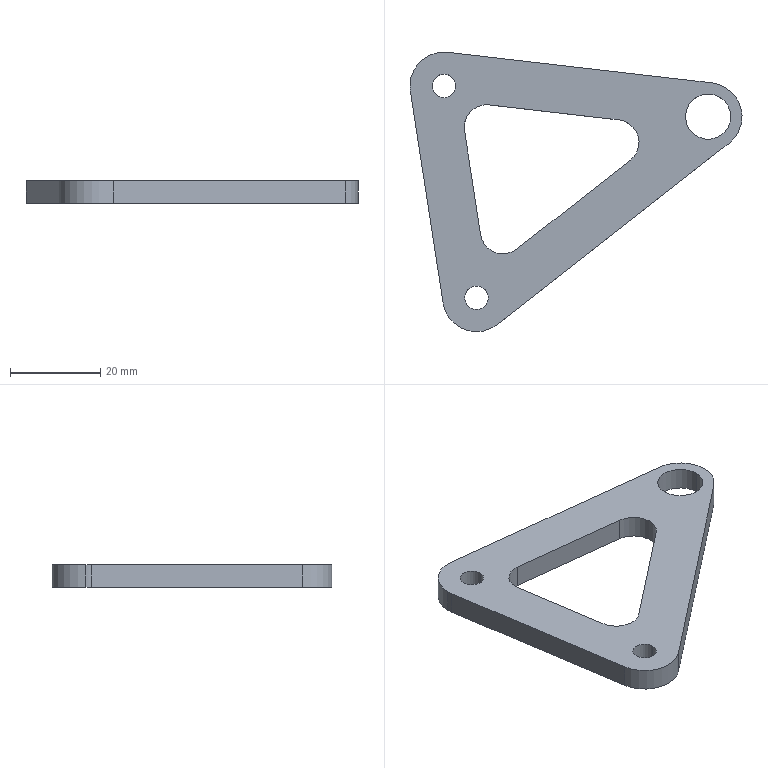Part | SolidWorks | features Extrusion 1 | 1 solid | 22 faces | box 73.414 x 61.829 x 5 mm | volume 9310 mm3 | cylinder 14 | plane 8 | commonest cylinder face diameters 10 x6 5.2 x4 15 x4
STEP:
#1=CARTESIAN_POINT('',(10.08,-4.188,5.));
#2=VERTEX_POINT('',#1);
#3=CARTESIAN_POINT('',(4.505,-9.155,5.));
#4=VERTEX_POINT('',#3);
#5=CARTESIAN_POINT('',(9.505,-9.155,5.));
#6=DIRECTION('',(0.,0.,1.));
#7=DIRECTION('',(-1.,0.,0.));
#8=AXIS2_PLACEMENT_3D('',#5,#6,#7);
#9=CIRCLE('',#8,5.);
#10=EDGE_CURVE('',#2,#4,#9,.T.);
#11=ORIENTED_EDGE('',*,*,#10,.T.);
#12=CARTESIAN_POINT('',(4.505,-9.155,0.));
#13=VERTEX_POINT('',#12);
#14=CARTESIAN_POINT('',(4.505,-9.155,5.));
#15=DIRECTION('',(0.,0.,-1.));
#16=VECTOR('',#15,1000.);
#17=LINE('',#14,#16);
#18=EDGE_CURVE('',#4,#13,#17,.T.);
#19=ORIENTED_EDGE('',*,*,#18,.T.);
#20=CARTESIAN_POINT('',(10.08,-4.188,0.));
#21=VERTEX_POINT('',#20);
#22=CARTESIAN_POINT('',(9.505,-9.155,0.));
#23=DIRECTION('',(0.,0.,1.));
#24=DIRECTION('',(-1.,0.,0.));
#25=AXIS2_PLACEMENT_3D('',#22,#23,#24);
#26=CIRCLE('',#25,5.);
#27=EDGE_CURVE('',#21,#13,#26,.T.);
#28=ORIENTED_EDGE('',*,*,#27,.F.);
#29=CARTESIAN_POINT('',(10.08,-4.188,5.));
#30=DIRECTION('',(0.,0.,-1.));
#31=VECTOR('',#30,1000.);
#32=LINE('',#29,#31);
#33=EDGE_CURVE('',#2,#21,#32,.T.);
#34=ORIENTED_EDGE('',*,*,#33,.F.);
#35=EDGE_LOOP('',(#11,#19,#28,#34));
#36=FACE_OUTER_BOUND('',#35,.T.);
#37=CARTESIAN_POINT('',(9.505,-9.155,5.));
#38=DIRECTION('',(0.,0.,-1.));
#39=DIRECTION('',(-1.,0.,0.));
#40=AXIS2_PLACEMENT_3D('',#37,#38,#39);
#41=CYLINDRICAL_SURFACE('',#40,5.);
#42=ADVANCED_FACE('',(#36),#41,.F.);
#43=CARTESIAN_POINT('',(-2.6,0.,5.));
#44=VERTEX_POINT('',#43);
#45=CARTESIAN_POINT('',(2.6,0.,5.));
#46=VERTEX_POINT('',#45);
#47=CARTESIAN_POINT('',(0.,0.,5.));
#48=DIRECTION('',(0.,0.,1.));
#49=DIRECTION('',(1.,0.,0.));
#50=AXIS2_PLACEMENT_3D('',#47,#48,#49);
#51=CIRCLE('',#50,2.6);
#52=EDGE_CURVE('',#44,#46,#51,.T.);
#53=ORIENTED_EDGE('',*,*,#52,.T.);
#54=CARTESIAN_POINT('',(2.6,0.,0.));
#55=VERTEX_POINT('',#54);
#56=CARTESIAN_POINT('',(2.6,0.,5.));
#57=DIRECTION('',(0.,0.,-1.));
#58=VECTOR('',#57,1000.);
#59=LINE('',#56,#58);
#60=EDGE_CURVE('',#46,#55,#59,.T.);
#61=ORIENTED_EDGE('',*,*,#60,.T.);
#62=CARTESIAN_POINT('',(-2.6,0.,0.));
#63=VERTEX_POINT('',#62);
#64=CARTESIAN_POINT('',(0.,0.,0.));
#65=DIRECTION('',(0.,0.,1.));
#66=DIRECTION('',(1.,0.,0.));
#67=AXIS2_PLACEMENT_3D('',#64,#65,#66);
#68=CIRCLE('',#67,2.6);
#69=EDGE_CURVE('',#63,#55,#68,.T.);
#70=ORIENTED_EDGE('',*,*,#69,.F.);
#71=CARTESIAN_POINT('',(-2.6,0.,5.));
#72=DIRECTION('',(0.,0.,-1.));
#73=VECTOR('',#72,1000.);
#74=LINE('',#71,#73);
#75=EDGE_CURVE('',#44,#63,#74,.T.);
#76=ORIENTED_EDGE('',*,*,#75,.F.);
#77=EDGE_LOOP('',(#53,#61,#70,#76));
#78=FACE_OUTER_BOUND('',#77,.T.);
#79=CARTESIAN_POINT('',(0.,0.,5.));
#80=DIRECTION('',(0.,0.,-1.));
#81=DIRECTION('',(-1.,0.,0.));
#82=AXIS2_PLACEMENT_3D('',#79,#80,#81);
#83=CYLINDRICAL_SURFACE('',#82,2.6);
#84=ADVANCED_FACE('',(#78),#83,.F.);
#85=CARTESIAN_POINT('',(53.414,-6.768,5.));
#86=VERTEX_POINT('',#85);
#87=CARTESIAN_POINT('',(63.414,-6.768,5.));
#88=VERTEX_POINT('',#87);
#89=CARTESIAN_POINT('',(58.414,-6.768,5.));
#90=DIRECTION('',(0.,0.,1.));
#91=DIRECTION('',(1.,0.,0.));
#92=AXIS2_PLACEMENT_3D('',#89,#90,#91);
#93=CIRCLE('',#92,5.);
#94=EDGE_CURVE('',#86,#88,#93,.T.);
#95=ORIENTED_EDGE('',*,*,#94,.T.);
#96=CARTESIAN_POINT('',(63.414,-6.768,0.));
#97=VERTEX_POINT('',#96);
#98=CARTESIAN_POINT('',(63.414,-6.768,5.));
#99=DIRECTION('',(0.,0.,-1.));
#100=VECTOR('',#99,1000.);
#101=LINE('',#98,#100);
#102=EDGE_CURVE('',#88,#97,#101,.T.);
#103=ORIENTED_EDGE('',*,*,#102,.T.);
#104=CARTESIAN_POINT('',(53.414,-6.768,0.));
#105=VERTEX_POINT('',#104);
#106=CARTESIAN_POINT('',(58.414,-6.768,0.));
#107=DIRECTION('',(0.,0.,1.));
#108=DIRECTION('',(1.,0.,0.));
#109=AXIS2_PLACEMENT_3D('',#106,#107,#108);
#110=CIRCLE('',#109,5.);
#111=EDGE_CURVE('',#105,#97,#110,.T.);
#112=ORIENTED_EDGE('',*,*,#111,.F.);
#113=CARTESIAN_POINT('',(53.414,-6.768,5.));
#114=DIRECTION('',(0.,0.,-1.));
#115=VECTOR('',#114,1000.);
#116=LINE('',#113,#115);
#117=EDGE_CURVE('',#86,#105,#116,.T.);
#118=ORIENTED_EDGE('',*,*,#117,.F.);
#119=EDGE_LOOP('',(#95,#103,#112,#118));
#120=FACE_OUTER_BOUND('',#119,.T.);
#121=CARTESIAN_POINT('',(58.414,-6.768,5.));
#122=DIRECTION('',(0.,0.,-1.));
#123=DIRECTION('',(-1.,0.,0.));
#124=AXIS2_PLACEMENT_3D('',#121,#122,#123);
#125=CYLINDRICAL_SURFACE('',#124,5.);
#126=ADVANCED_FACE('',(#120),#125,.F.);
#127=CARTESIAN_POINT('',(4.614,-46.829,5.));
#128=VERTEX_POINT('',#127);
#129=CARTESIAN_POINT('',(9.814,-46.829,5.));
#130=VERTEX_POINT('',#129);
#131=CARTESIAN_POINT('',(7.214,-46.829,5.));
#132=DIRECTION('',(0.,0.,1.));
#133=DIRECTION('',(1.,0.,0.));
#134=AXIS2_PLACEMENT_3D('',#131,#132,#133);
#135=CIRCLE('',#134,2.6);
#136=EDGE_CURVE('',#128,#130,#135,.T.);
#137=ORIENTED_EDGE('',*,*,#136,.T.);
#138=CARTESIAN_POINT('',(9.814,-46.829,0.));
#139=VERTEX_POINT('',#138);
#140=CARTESIAN_POINT('',(9.814,-46.829,5.));
#141=DIRECTION('',(0.,0.,-1.));
#142=VECTOR('',#141,1000.);
#143=LINE('',#140,#142);
#144=EDGE_CURVE('',#130,#139,#143,.T.);
#145=ORIENTED_EDGE('',*,*,#144,.T.);
#146=CARTESIAN_POINT('',(4.614,-46.829,0.));
#147=VERTEX_POINT('',#146);
#148=CARTESIAN_POINT('',(7.214,-46.829,0.));
#149=DIRECTION('',(0.,0.,1.));
#150=DIRECTION('',(1.,0.,0.));
#151=AXIS2_PLACEMENT_3D('',#148,#149,#150);
#152=CIRCLE('',#151,2.6);
#153=EDGE_CURVE('',#147,#139,#152,.T.);
#154=ORIENTED_EDGE('',*,*,#153,.F.);
#155=CARTESIAN_POINT('',(4.614,-46.829,5.));
#156=DIRECTION('',(0.,0.,-1.));
#157=VECTOR('',#156,1000.);
#158=LINE('',#155,#157);
#159=EDGE_CURVE('',#128,#147,#158,.T.);
#160=ORIENTED_EDGE('',*,*,#159,.F.);
#161=EDGE_LOOP('',(#137,#145,#154,#160));
#162=FACE_OUTER_BOUND('',#161,.T.);
#163=CARTESIAN_POINT('',(7.214,-46.829,5.));
#164=DIRECTION('',(0.,0.,-1.));
#165=DIRECTION('',(-1.,0.,0.));
#166=AXIS2_PLACEMENT_3D('',#163,#164,#165);
#167=CYLINDRICAL_SURFACE('',#166,2.6);
#168=ADVANCED_FACE('',(#162),#167,.F.);
#169=CARTESIAN_POINT('',(-7.5,0.,5.));
#170=VERTEX_POINT('',#169);
#171=CARTESIAN_POINT('',(-7.413,-1.142,5.));
#172=VERTEX_POINT('',#171);
#173=CARTESIAN_POINT('',(0.,0.,5.));
#174=DIRECTION('',(0.,0.,1.));
#175=DIRECTION('',(1.,0.,0.));
#176=AXIS2_PLACEMENT_3D('',#173,#174,#175);
#177=CIRCLE('',#176,7.5);
#178=EDGE_CURVE('',#170,#172,#177,.T.);
#179=ORIENTED_EDGE('',*,*,#178,.F.);
#180=CARTESIAN_POINT('',(-7.5,0.,0.));
#181=VERTEX_POINT('',#180);
#182=CARTESIAN_POINT('',(-7.5,0.,5.));
#183=DIRECTION('',(0.,0.,-1.));
#184=VECTOR('',#183,1000.);
#185=LINE('',#182,#184);
#186=EDGE_CURVE('',#170,#181,#185,.T.);
#187=ORIENTED_EDGE('',*,*,#186,.T.);
#188=CARTESIAN_POINT('',(-7.413,-1.142,0.));
#189=VERTEX_POINT('',#188);
#190=CARTESIAN_POINT('',(0.,0.,0.));
#191=DIRECTION('',(0.,0.,1.));
#192=DIRECTION('',(1.,0.,0.));
#193=AXIS2_PLACEMENT_3D('',#190,#191,#192);
#194=CIRCLE('',#193,7.5);
#195=EDGE_CURVE('',#181,#189,#194,.T.);
#196=ORIENTED_EDGE('',*,*,#195,.T.);
#197=CARTESIAN_POINT('',(-7.413,-1.142,5.));
#198=DIRECTION('',(0.,0.,-1.));
#199=VECTOR('',#198,1000.);
#200=LINE('',#197,#199);
#201=EDGE_CURVE('',#172,#189,#200,.T.);
#202=ORIENTED_EDGE('',*,*,#201,.F.);
#203=EDGE_LOOP('',(#179,#187,#196,#202));
#204=FACE_OUTER_BOUND('',#203,.T.);
#205=CARTESIAN_POINT('',(0.,0.,5.));
#206=DIRECTION('',(0.,0.,-1.));
#207=DIRECTION('',(-1.,0.,0.));
#208=AXIS2_PLACEMENT_3D('',#205,#206,#207);
#209=CYLINDRICAL_SURFACE('',#208,7.5);
#210=ADVANCED_FACE('',(#204),#209,.T.);
#211=ORIENTED_EDGE('',*,*,#94,.F.);
#212=CARTESIAN_POINT('',(58.414,-6.768,5.));
#213=DIRECTION('',(0.,0.,1.));
#214=DIRECTION('',(1.,0.,0.));
#215=AXIS2_PLACEMENT_3D('',#212,#213,#214);
#216=CIRCLE('',#215,5.);
#217=EDGE_CURVE('',#88,#86,#216,.T.);
#218=ORIENTED_EDGE('',*,*,#217,.F.);
#219=EDGE_LOOP('',(#211,#218));
#220=FACE_BOUND('',#219,.T.);
#221=CARTESIAN_POINT('',(63.036,-12.674,5.));
#222=VERTEX_POINT('',#221);
#223=CARTESIAN_POINT('',(59.277,0.6826,5.));
#224=VERTEX_POINT('',#223);
#225=CARTESIAN_POINT('',(58.414,-6.768,5.));
#226=DIRECTION('',(0.,0.,1.));
#227=DIRECTION('',(1.,0.,0.));
#228=AXIS2_PLACEMENT_3D('',#225,#226,#227);
#229=CIRCLE('',#228,7.5);
#230=EDGE_CURVE('',#222,#224,#229,.T.);
#231=ORIENTED_EDGE('',*,*,#230,.T.);
#232=CARTESIAN_POINT('',(0.8631,7.45,5.));
#233=VERTEX_POINT('',#232);
#234=CARTESIAN_POINT('',(59.277,0.6826,5.));
#235=DIRECTION('',(-0.9934,0.1151,0.));
#236=VECTOR('',#235,1000.);
#237=LINE('',#234,#236);
#238=EDGE_CURVE('',#224,#233,#237,.T.);
#239=ORIENTED_EDGE('',*,*,#238,.T.);
#240=CARTESIAN_POINT('',(0.,0.,5.));
#241=DIRECTION('',(0.,0.,1.));
#242=DIRECTION('',(1.,0.,0.));
#243=AXIS2_PLACEMENT_3D('',#240,#241,#242);
#244=CIRCLE('',#243,7.5);
#245=EDGE_CURVE('',#233,#170,#244,.T.);
#246=ORIENTED_EDGE('',*,*,#245,.T.);
#247=ORIENTED_EDGE('',*,*,#178,.T.);
#248=CARTESIAN_POINT('',(-0.1986,-47.971,5.));
#249=VERTEX_POINT('',#248);
#250=CARTESIAN_POINT('',(-7.413,-1.142,5.));
#251=DIRECTION('',(0.1523,-0.9883,0.));
#252=VECTOR('',#251,1000.);
#253=LINE('',#250,#252);
#254=EDGE_CURVE('',#172,#249,#253,.T.);
#255=ORIENTED_EDGE('',*,*,#254,.T.);
#256=CARTESIAN_POINT('',(11.836,-52.736,5.));
#257=VERTEX_POINT('',#256);
#258=CARTESIAN_POINT('',(7.214,-46.829,5.));
#259=DIRECTION('',(0.,0.,1.));
#260=DIRECTION('',(1.,0.,0.));
#261=AXIS2_PLACEMENT_3D('',#258,#259,#260);
#262=CIRCLE('',#261,7.5);
#263=EDGE_CURVE('',#249,#257,#262,.T.);
#264=ORIENTED_EDGE('',*,*,#263,.T.);
#265=CARTESIAN_POINT('',(11.836,-52.736,5.));
#266=DIRECTION('',(0.7876,0.6162,0.));
#267=VECTOR('',#266,1000.);
#268=LINE('',#265,#267);
#269=EDGE_CURVE('',#257,#222,#268,.T.);
#270=ORIENTED_EDGE('',*,*,#269,.T.);
#271=EDGE_LOOP('',(#231,#239,#246,#247,#255,#264,#270));
#272=FACE_OUTER_BOUND('',#271,.T.);
#273=ORIENTED_EDGE('',*,*,#136,.F.);
#274=CARTESIAN_POINT('',(7.214,-46.829,5.));
#275=DIRECTION('',(0.,0.,1.));
#276=DIRECTION('',(1.,0.,0.));
#277=AXIS2_PLACEMENT_3D('',#274,#275,#276);
#278=CIRCLE('',#277,2.6);
#279=EDGE_CURVE('',#130,#128,#278,.T.);
#280=ORIENTED_EDGE('',*,*,#279,.F.);
#281=EDGE_LOOP('',(#273,#280));
#282=FACE_BOUND('',#281,.T.);
#283=ORIENTED_EDGE('',*,*,#52,.F.);
#284=CARTESIAN_POINT('',(0.,0.,5.));
#285=DIRECTION('',(0.,0.,1.));
#286=DIRECTION('',(1.,0.,0.));
#287=AXIS2_PLACEMENT_3D('',#284,#285,#286);
#288=CIRCLE('',#287,2.6);
#289=EDGE_CURVE('',#46,#44,#288,.T.);
#290=ORIENTED_EDGE('',*,*,#289,.F.);
#291=EDGE_LOOP('',(#283,#290));
#292=FACE_BOUND('',#291,.T.);
#293=CARTESIAN_POINT('',(16.122,-36.05,5.));
#294=VERTEX_POINT('',#293);
#295=CARTESIAN_POINT('',(41.222,-16.41,5.));
#296=VERTEX_POINT('',#295);
#297=CARTESIAN_POINT('',(16.122,-36.05,5.));
#298=DIRECTION('',(0.7876,0.6162,0.));
#299=VECTOR('',#298,1000.);
#300=LINE('',#297,#299);
#301=EDGE_CURVE('',#294,#296,#300,.T.);
#302=ORIENTED_EDGE('',*,*,#301,.F.);
#303=CARTESIAN_POINT('',(8.099,-32.873,5.));
#304=VERTEX_POINT('',#303);
#305=CARTESIAN_POINT('',(13.041,-32.112,5.));
#306=DIRECTION('',(0.,0.,1.));
#307=DIRECTION('',(-1.,0.,0.));
#308=AXIS2_PLACEMENT_3D('',#305,#306,#307);
#309=CIRCLE('',#308,5.);
#310=EDGE_CURVE('',#304,#294,#309,.T.);
#311=ORIENTED_EDGE('',*,*,#310,.F.);
#312=CARTESIAN_POINT('',(4.563,-9.916,5.));
#313=VERTEX_POINT('',#312);
#314=CARTESIAN_POINT('',(4.563,-9.916,5.));
#315=DIRECTION('',(0.1523,-0.9883,0.));
#316=VECTOR('',#315,1000.);
#317=LINE('',#314,#316);
#318=EDGE_CURVE('',#313,#304,#317,.T.);
#319=ORIENTED_EDGE('',*,*,#318,.F.);
#320=CARTESIAN_POINT('',(9.505,-9.155,5.));
#321=DIRECTION('',(0.,0.,1.));
#322=DIRECTION('',(-1.,0.,0.));
#323=AXIS2_PLACEMENT_3D('',#320,#321,#322);
#324=CIRCLE('',#323,5.);
#325=EDGE_CURVE('',#4,#313,#324,.T.);
#326=ORIENTED_EDGE('',*,*,#325,.F.);
#327=ORIENTED_EDGE('',*,*,#10,.F.);
#328=CARTESIAN_POINT('',(38.717,-7.506,5.));
#329=VERTEX_POINT('',#328);
#330=CARTESIAN_POINT('',(38.717,-7.506,5.));
#331=DIRECTION('',(-0.9934,0.1151,0.));
#332=VECTOR('',#331,1000.);
#333=LINE('',#330,#332);
#334=EDGE_CURVE('',#329,#2,#333,.T.);
#335=ORIENTED_EDGE('',*,*,#334,.F.);
#336=CARTESIAN_POINT('',(38.141,-12.472,5.));
#337=DIRECTION('',(0.,0.,1.));
#338=DIRECTION('',(1.,0.,0.));
#339=AXIS2_PLACEMENT_3D('',#336,#337,#338);
#340=CIRCLE('',#339,5.);
#341=EDGE_CURVE('',#296,#329,#340,.T.);
#342=ORIENTED_EDGE('',*,*,#341,.F.);
#343=EDGE_LOOP('',(#302,#311,#319,#326,#327,#335,#342));
#344=FACE_BOUND('',#343,.T.);
#345=CARTESIAN_POINT('',(58.414,-6.768,5.));
#346=DIRECTION('',(0.,0.,1.));
#347=DIRECTION('',(1.,0.,0.));
#348=AXIS2_PLACEMENT_3D('',#345,#346,#347);
#349=PLANE('',#348);
#350=ADVANCED_FACE('',(#220,#272,#282,#292,#344),#349,.T.);
#351=ORIENTED_EDGE('',*,*,#69,.T.);
#352=CARTESIAN_POINT('',(0.,0.,0.));
#353=DIRECTION('',(0.,0.,1.));
#354=DIRECTION('',(1.,0.,0.));
#355=AXIS2_PLACEMENT_3D('',#352,#353,#354);
#356=CIRCLE('',#355,2.6);
#357=EDGE_CURVE('',#55,#63,#356,.T.);
#358=ORIENTED_EDGE('',*,*,#357,.T.);
#359=EDGE_LOOP('',(#351,#358));
#360=FACE_BOUND('',#359,.T.);
#361=ORIENTED_EDGE('',*,*,#111,.T.);
#362=CARTESIAN_POINT('',(58.414,-6.768,0.));
#363=DIRECTION('',(0.,0.,1.));
#364=DIRECTION('',(1.,0.,0.));
#365=AXIS2_PLACEMENT_3D('',#362,#363,#364);
#366=CIRCLE('',#365,5.);
#367=EDGE_CURVE('',#97,#105,#366,.T.);
#368=ORIENTED_EDGE('',*,*,#367,.T.);
#369=EDGE_LOOP('',(#361,#368));
#370=FACE_BOUND('',#369,.T.);
#371=ORIENTED_EDGE('',*,*,#153,.T.);
#372=CARTESIAN_POINT('',(7.214,-46.829,0.));
#373=DIRECTION('',(0.,0.,1.));
#374=DIRECTION('',(1.,0.,0.));
#375=AXIS2_PLACEMENT_3D('',#372,#373,#374);
#376=CIRCLE('',#375,2.6);
#377=EDGE_CURVE('',#139,#147,#376,.T.);
#378=ORIENTED_EDGE('',*,*,#377,.T.);
#379=EDGE_LOOP('',(#371,#378));
#380=FACE_BOUND('',#379,.T.);
#381=CARTESIAN_POINT('',(63.036,-12.674,0.));
#382=VERTEX_POINT('',#381);
#383=CARTESIAN_POINT('',(59.277,0.6826,0.));
#384=VERTEX_POINT('',#383);
#385=CARTESIAN_POINT('',(58.414,-6.768,0.));
#386=DIRECTION('',(0.,0.,1.));
#387=DIRECTION('',(1.,0.,0.));
#388=AXIS2_PLACEMENT_3D('',#385,#386,#387);
#389=CIRCLE('',#388,7.5);
#390=EDGE_CURVE('',#382,#384,#389,.T.);
#391=ORIENTED_EDGE('',*,*,#390,.F.);
#392=CARTESIAN_POINT('',(11.836,-52.736,0.));
#393=VERTEX_POINT('',#392);
#394=CARTESIAN_POINT('',(11.836,-52.736,0.));
#395=DIRECTION('',(0.7876,0.6162,0.));
#396=VECTOR('',#395,1000.);
#397=LINE('',#394,#396);
#398=EDGE_CURVE('',#393,#382,#397,.T.);
#399=ORIENTED_EDGE('',*,*,#398,.F.);
#400=CARTESIAN_POINT('',(-0.1986,-47.971,0.));
#401=VERTEX_POINT('',#400);
#402=CARTESIAN_POINT('',(7.214,-46.829,0.));
#403=DIRECTION('',(0.,0.,1.));
#404=DIRECTION('',(1.,0.,0.));
#405=AXIS2_PLACEMENT_3D('',#402,#403,#404);
#406=CIRCLE('',#405,7.5);
#407=EDGE_CURVE('',#401,#393,#406,.T.);
#408=ORIENTED_EDGE('',*,*,#407,.F.);
#409=CARTESIAN_POINT('',(-7.413,-1.142,0.));
#410=DIRECTION('',(0.1523,-0.9883,0.));
#411=VECTOR('',#410,1000.);
#412=LINE('',#409,#411);
#413=EDGE_CURVE('',#189,#401,#412,.T.);
#414=ORIENTED_EDGE('',*,*,#413,.F.);
#415=ORIENTED_EDGE('',*,*,#195,.F.);
#416=CARTESIAN_POINT('',(0.8631,7.45,0.));
#417=VERTEX_POINT('',#416);
#418=CARTESIAN_POINT('',(0.,0.,0.));
#419=DIRECTION('',(0.,0.,1.));
#420=DIRECTION('',(1.,0.,0.));
#421=AXIS2_PLACEMENT_3D('',#418,#419,#420);
#422=CIRCLE('',#421,7.5);
#423=EDGE_CURVE('',#417,#181,#422,.T.);
#424=ORIENTED_EDGE('',*,*,#423,.F.);
#425=CARTESIAN_POINT('',(59.277,0.6826,0.));
#426=DIRECTION('',(-0.9934,0.1151,0.));
#427=VECTOR('',#426,1000.);
#428=LINE('',#425,#427);
#429=EDGE_CURVE('',#384,#417,#428,.T.);
#430=ORIENTED_EDGE('',*,*,#429,.F.);
#431=EDGE_LOOP('',(#391,#399,#408,#414,#415,#424,#430));
#432=FACE_OUTER_BOUND('',#431,.T.);
#433=CARTESIAN_POINT('',(8.099,-32.873,0.));
#434=VERTEX_POINT('',#433);
#435=CARTESIAN_POINT('',(16.122,-36.05,0.));
#436=VERTEX_POINT('',#435);
#437=CARTESIAN_POINT('',(13.041,-32.112,0.));
#438=DIRECTION('',(0.,0.,1.));
#439=DIRECTION('',(-1.,0.,0.));
#440=AXIS2_PLACEMENT_3D('',#437,#438,#439);
#441=CIRCLE('',#440,5.);
#442=EDGE_CURVE('',#434,#436,#441,.T.);
#443=ORIENTED_EDGE('',*,*,#442,.T.);
#444=CARTESIAN_POINT('',(41.222,-16.41,0.));
#445=VERTEX_POINT('',#444);
#446=CARTESIAN_POINT('',(16.122,-36.05,0.));
#447=DIRECTION('',(0.7876,0.6162,0.));
#448=VECTOR('',#447,1000.);
#449=LINE('',#446,#448);
#450=EDGE_CURVE('',#436,#445,#449,.T.);
#451=ORIENTED_EDGE('',*,*,#450,.T.);
#452=CARTESIAN_POINT('',(38.717,-7.506,0.));
#453=VERTEX_POINT('',#452);
#454=CARTESIAN_POINT('',(38.141,-12.472,0.));
#455=DIRECTION('',(0.,0.,1.));
#456=DIRECTION('',(1.,0.,0.));
#457=AXIS2_PLACEMENT_3D('',#454,#455,#456);
#458=CIRCLE('',#457,5.);
#459=EDGE_CURVE('',#445,#453,#458,.T.);
#460=ORIENTED_EDGE('',*,*,#459,.T.);
#461=CARTESIAN_POINT('',(38.717,-7.506,0.));
#462=DIRECTION('',(-0.9934,0.1151,0.));
#463=VECTOR('',#462,1000.);
#464=LINE('',#461,#463);
#465=EDGE_CURVE('',#453,#21,#464,.T.);
#466=ORIENTED_EDGE('',*,*,#465,.T.);
#467=ORIENTED_EDGE('',*,*,#27,.T.);
#468=CARTESIAN_POINT('',(4.563,-9.916,0.));
#469=VERTEX_POINT('',#468);
#470=CARTESIAN_POINT('',(9.505,-9.155,0.));
#471=DIRECTION('',(0.,0.,1.));
#472=DIRECTION('',(-1.,0.,0.));
#473=AXIS2_PLACEMENT_3D('',#470,#471,#472);
#474=CIRCLE('',#473,5.);
#475=EDGE_CURVE('',#13,#469,#474,.T.);
#476=ORIENTED_EDGE('',*,*,#475,.T.);
#477=CARTESIAN_POINT('',(4.563,-9.916,0.));
#478=DIRECTION('',(0.1523,-0.9883,0.));
#479=VECTOR('',#478,1000.);
#480=LINE('',#477,#479);
#481=EDGE_CURVE('',#469,#434,#480,.T.);
#482=ORIENTED_EDGE('',*,*,#481,.T.);
#483=EDGE_LOOP('',(#443,#451,#460,#466,#467,#476,#482));
#484=FACE_BOUND('',#483,.T.);
#485=CARTESIAN_POINT('',(58.414,-6.768,0.));
#486=DIRECTION('',(0.,0.,1.));
#487=DIRECTION('',(1.,0.,0.));
#488=AXIS2_PLACEMENT_3D('',#485,#486,#487);
#489=PLANE('',#488);
#490=ADVANCED_FACE('',(#360,#370,#380,#432,#484),#489,.F.);
#491=ORIENTED_EDGE('',*,*,#390,.T.);
#492=CARTESIAN_POINT('',(59.277,0.6826,5.));
#493=DIRECTION('',(0.,0.,-1.));
#494=VECTOR('',#493,1000.);
#495=LINE('',#492,#494);
#496=EDGE_CURVE('',#224,#384,#495,.T.);
#497=ORIENTED_EDGE('',*,*,#496,.F.);
#498=ORIENTED_EDGE('',*,*,#230,.F.);
#499=CARTESIAN_POINT('',(63.036,-12.674,5.));
#500=DIRECTION('',(0.,0.,-1.));
#501=VECTOR('',#500,1000.);
#502=LINE('',#499,#501);
#503=EDGE_CURVE('',#222,#382,#502,.T.);
#504=ORIENTED_EDGE('',*,*,#503,.T.);
#505=EDGE_LOOP('',(#491,#497,#498,#504));
#506=FACE_OUTER_BOUND('',#505,.T.);
#507=CARTESIAN_POINT('',(58.414,-6.768,5.));
#508=DIRECTION('',(0.,0.,-1.));
#509=DIRECTION('',(-1.,0.,0.));
#510=AXIS2_PLACEMENT_3D('',#507,#508,#509);
#511=CYLINDRICAL_SURFACE('',#510,7.5);
#512=ADVANCED_FACE('',(#506),#511,.T.);
#513=ORIENTED_EDGE('',*,*,#429,.T.);
#514=CARTESIAN_POINT('',(0.8631,7.45,5.));
#515=DIRECTION('',(0.,0.,-1.));
#516=VECTOR('',#515,1000.);
#517=LINE('',#514,#516);
#518=EDGE_CURVE('',#233,#417,#517,.T.);
#519=ORIENTED_EDGE('',*,*,#518,.F.);
#520=ORIENTED_EDGE('',*,*,#238,.F.);
#521=ORIENTED_EDGE('',*,*,#496,.T.);
#522=EDGE_LOOP('',(#513,#519,#520,#521));
#523=FACE_OUTER_BOUND('',#522,.T.);
#524=CARTESIAN_POINT('',(59.277,0.6826,5.));
#525=DIRECTION('',(-0.1151,-0.9934,0.));
#526=DIRECTION('',(0.9934,-0.1151,0.));
#527=AXIS2_PLACEMENT_3D('',#524,#525,#526);
#528=PLANE('',#527);
#529=ADVANCED_FACE('',(#523),#528,.F.);
#530=ORIENTED_EDGE('',*,*,#186,.F.);
#531=ORIENTED_EDGE('',*,*,#245,.F.);
#532=ORIENTED_EDGE('',*,*,#518,.T.);
#533=ORIENTED_EDGE('',*,*,#423,.T.);
#534=EDGE_LOOP('',(#530,#531,#532,#533));
#535=FACE_OUTER_BOUND('',#534,.T.);
#536=CARTESIAN_POINT('',(0.,0.,5.));
#537=DIRECTION('',(0.,0.,-1.));
#538=DIRECTION('',(-1.,0.,0.));
#539=AXIS2_PLACEMENT_3D('',#536,#537,#538);
#540=CYLINDRICAL_SURFACE('',#539,7.5);
#541=ADVANCED_FACE('',(#535),#540,.T.);
#542=ORIENTED_EDGE('',*,*,#413,.T.);
#543=CARTESIAN_POINT('',(-0.1986,-47.971,5.));
#544=DIRECTION('',(0.,0.,-1.));
#545=VECTOR('',#544,1000.);
#546=LINE('',#543,#545);
#547=EDGE_CURVE('',#249,#401,#546,.T.);
#548=ORIENTED_EDGE('',*,*,#547,.F.);
#549=ORIENTED_EDGE('',*,*,#254,.F.);
#550=ORIENTED_EDGE('',*,*,#201,.T.);
#551=EDGE_LOOP('',(#542,#548,#549,#550));
#552=FACE_OUTER_BOUND('',#551,.T.);
#553=CARTESIAN_POINT('',(-7.413,-1.142,5.));
#554=DIRECTION('',(0.9883,0.1523,0.));
#555=DIRECTION('',(-0.1523,0.9883,0.));
#556=AXIS2_PLACEMENT_3D('',#553,#554,#555);
#557=PLANE('',#556);
#558=ADVANCED_FACE('',(#552),#557,.F.);
#559=ORIENTED_EDGE('',*,*,#407,.T.);
#560=CARTESIAN_POINT('',(11.836,-52.736,5.));
#561=DIRECTION('',(0.,0.,-1.));
#562=VECTOR('',#561,1000.);
#563=LINE('',#560,#562);
#564=EDGE_CURVE('',#257,#393,#563,.T.);
#565=ORIENTED_EDGE('',*,*,#564,.F.);
#566=ORIENTED_EDGE('',*,*,#263,.F.);
#567=ORIENTED_EDGE('',*,*,#547,.T.);
#568=EDGE_LOOP('',(#559,#565,#566,#567));
#569=FACE_OUTER_BOUND('',#568,.T.);
#570=CARTESIAN_POINT('',(7.214,-46.829,5.));
#571=DIRECTION('',(0.,0.,-1.));
#572=DIRECTION('',(-1.,0.,0.));
#573=AXIS2_PLACEMENT_3D('',#570,#571,#572);
#574=CYLINDRICAL_SURFACE('',#573,7.5);
#575=ADVANCED_FACE('',(#569),#574,.T.);
#576=ORIENTED_EDGE('',*,*,#398,.T.);
#577=ORIENTED_EDGE('',*,*,#503,.F.);
#578=ORIENTED_EDGE('',*,*,#269,.F.);
#579=ORIENTED_EDGE('',*,*,#564,.T.);
#580=EDGE_LOOP('',(#576,#577,#578,#579));
#581=FACE_OUTER_BOUND('',#580,.T.);
#582=CARTESIAN_POINT('',(11.836,-52.736,5.));
#583=DIRECTION('',(-0.6162,0.7876,0.));
#584=DIRECTION('',(-0.7876,-0.6162,0.));
#585=AXIS2_PLACEMENT_3D('',#582,#583,#584);
#586=PLANE('',#585);
#587=ADVANCED_FACE('',(#581),#586,.F.);
#588=ORIENTED_EDGE('',*,*,#144,.F.);
#589=ORIENTED_EDGE('',*,*,#279,.T.);
#590=ORIENTED_EDGE('',*,*,#159,.T.);
#591=ORIENTED_EDGE('',*,*,#377,.F.);
#592=EDGE_LOOP('',(#588,#589,#590,#591));
#593=FACE_OUTER_BOUND('',#592,.T.);
#594=CARTESIAN_POINT('',(7.214,-46.829,5.));
#595=DIRECTION('',(0.,0.,-1.));
#596=DIRECTION('',(-1.,0.,0.));
#597=AXIS2_PLACEMENT_3D('',#594,#595,#596);
#598=CYLINDRICAL_SURFACE('',#597,2.6);
#599=ADVANCED_FACE('',(#593),#598,.F.);
#600=ORIENTED_EDGE('',*,*,#102,.F.);
#601=ORIENTED_EDGE('',*,*,#217,.T.);
#602=ORIENTED_EDGE('',*,*,#117,.T.);
#603=ORIENTED_EDGE('',*,*,#367,.F.);
#604=EDGE_LOOP('',(#600,#601,#602,#603));
#605=FACE_OUTER_BOUND('',#604,.T.);
#606=CARTESIAN_POINT('',(58.414,-6.768,5.));
#607=DIRECTION('',(0.,0.,-1.));
#608=DIRECTION('',(-1.,0.,0.));
#609=AXIS2_PLACEMENT_3D('',#606,#607,#608);
#610=CYLINDRICAL_SURFACE('',#609,5.);
#611=ADVANCED_FACE('',(#605),#610,.F.);
#612=ORIENTED_EDGE('',*,*,#60,.F.);
#613=ORIENTED_EDGE('',*,*,#289,.T.);
#614=ORIENTED_EDGE('',*,*,#75,.T.);
#615=ORIENTED_EDGE('',*,*,#357,.F.);
#616=EDGE_LOOP('',(#612,#613,#614,#615));
#617=FACE_OUTER_BOUND('',#616,.T.);
#618=CARTESIAN_POINT('',(0.,0.,5.));
#619=DIRECTION('',(0.,0.,-1.));
#620=DIRECTION('',(-1.,0.,0.));
#621=AXIS2_PLACEMENT_3D('',#618,#619,#620);
#622=CYLINDRICAL_SURFACE('',#621,2.6);
#623=ADVANCED_FACE('',(#617),#622,.F.);
#624=ORIENTED_EDGE('',*,*,#442,.F.);
#625=CARTESIAN_POINT('',(8.099,-32.873,5.));
#626=DIRECTION('',(0.,0.,-1.));
#627=VECTOR('',#626,1000.);
#628=LINE('',#625,#627);
#629=EDGE_CURVE('',#304,#434,#628,.T.);
#630=ORIENTED_EDGE('',*,*,#629,.F.);
#631=ORIENTED_EDGE('',*,*,#310,.T.);
#632=CARTESIAN_POINT('',(16.122,-36.05,5.));
#633=DIRECTION('',(0.,0.,-1.));
#634=VECTOR('',#633,1000.);
#635=LINE('',#632,#634);
#636=EDGE_CURVE('',#294,#436,#635,.T.);
#637=ORIENTED_EDGE('',*,*,#636,.T.);
#638=EDGE_LOOP('',(#624,#630,#631,#637));
#639=FACE_OUTER_BOUND('',#638,.T.);
#640=CARTESIAN_POINT('',(13.041,-32.112,5.));
#641=DIRECTION('',(0.,0.,-1.));
#642=DIRECTION('',(-1.,0.,0.));
#643=AXIS2_PLACEMENT_3D('',#640,#641,#642);
#644=CYLINDRICAL_SURFACE('',#643,5.);
#645=ADVANCED_FACE('',(#639),#644,.F.);
#646=ORIENTED_EDGE('',*,*,#450,.F.);
#647=ORIENTED_EDGE('',*,*,#636,.F.);
#648=ORIENTED_EDGE('',*,*,#301,.T.);
#649=CARTESIAN_POINT('',(41.222,-16.41,5.));
#650=DIRECTION('',(0.,0.,-1.));
#651=VECTOR('',#650,1000.);
#652=LINE('',#649,#651);
#653=EDGE_CURVE('',#296,#445,#652,.T.);
#654=ORIENTED_EDGE('',*,*,#653,.T.);
#655=EDGE_LOOP('',(#646,#647,#648,#654));
#656=FACE_OUTER_BOUND('',#655,.T.);
#657=CARTESIAN_POINT('',(16.122,-36.05,5.));
#658=DIRECTION('',(-0.6162,0.7876,0.));
#659=DIRECTION('',(-0.7876,-0.6162,0.));
#660=AXIS2_PLACEMENT_3D('',#657,#658,#659);
#661=PLANE('',#660);
#662=ADVANCED_FACE('',(#656),#661,.T.);
#663=ORIENTED_EDGE('',*,*,#459,.F.);
#664=ORIENTED_EDGE('',*,*,#653,.F.);
#665=ORIENTED_EDGE('',*,*,#341,.T.);
#666=CARTESIAN_POINT('',(38.717,-7.506,5.));
#667=DIRECTION('',(0.,0.,-1.));
#668=VECTOR('',#667,1000.);
#669=LINE('',#666,#668);
#670=EDGE_CURVE('',#329,#453,#669,.T.);
#671=ORIENTED_EDGE('',*,*,#670,.T.);
#672=EDGE_LOOP('',(#663,#664,#665,#671));
#673=FACE_OUTER_BOUND('',#672,.T.);
#674=CARTESIAN_POINT('',(38.141,-12.472,5.));
#675=DIRECTION('',(0.,0.,-1.));
#676=DIRECTION('',(-1.,0.,0.));
#677=AXIS2_PLACEMENT_3D('',#674,#675,#676);
#678=CYLINDRICAL_SURFACE('',#677,5.);
#679=ADVANCED_FACE('',(#673),#678,.F.);
#680=ORIENTED_EDGE('',*,*,#465,.F.);
#681=ORIENTED_EDGE('',*,*,#670,.F.);
#682=ORIENTED_EDGE('',*,*,#334,.T.);
#683=ORIENTED_EDGE('',*,*,#33,.T.);
#684=EDGE_LOOP('',(#680,#681,#682,#683));
#685=FACE_OUTER_BOUND('',#684,.T.);
#686=CARTESIAN_POINT('',(38.717,-7.506,5.));
#687=DIRECTION('',(-0.1151,-0.9934,0.));
#688=DIRECTION('',(0.9934,-0.1151,0.));
#689=AXIS2_PLACEMENT_3D('',#686,#687,#688);
#690=PLANE('',#689);
#691=ADVANCED_FACE('',(#685),#690,.T.);
#692=ORIENTED_EDGE('',*,*,#18,.F.);
#693=ORIENTED_EDGE('',*,*,#325,.T.);
#694=CARTESIAN_POINT('',(4.563,-9.916,5.));
#695=DIRECTION('',(0.,0.,-1.));
#696=VECTOR('',#695,1000.);
#697=LINE('',#694,#696);
#698=EDGE_CURVE('',#313,#469,#697,.T.);
#699=ORIENTED_EDGE('',*,*,#698,.T.);
#700=ORIENTED_EDGE('',*,*,#475,.F.);
#701=EDGE_LOOP('',(#692,#693,#699,#700));
#702=FACE_OUTER_BOUND('',#701,.T.);
#703=CARTESIAN_POINT('',(9.505,-9.155,5.));
#704=DIRECTION('',(0.,0.,-1.));
#705=DIRECTION('',(-1.,0.,0.));
#706=AXIS2_PLACEMENT_3D('',#703,#704,#705);
#707=CYLINDRICAL_SURFACE('',#706,5.);
#708=ADVANCED_FACE('',(#702),#707,.F.);
#709=ORIENTED_EDGE('',*,*,#481,.F.);
#710=ORIENTED_EDGE('',*,*,#698,.F.);
#711=ORIENTED_EDGE('',*,*,#318,.T.);
#712=ORIENTED_EDGE('',*,*,#629,.T.);
#713=EDGE_LOOP('',(#709,#710,#711,#712));
#714=FACE_OUTER_BOUND('',#713,.T.);
#715=CARTESIAN_POINT('',(4.563,-9.916,5.));
#716=DIRECTION('',(0.9883,0.1523,0.));
#717=DIRECTION('',(-0.1523,0.9883,0.));
#718=AXIS2_PLACEMENT_3D('',#715,#716,#717);
#719=PLANE('',#718);
#720=ADVANCED_FACE('',(#714),#719,.T.);
#721=CLOSED_SHELL('',(#42,#84,#126,#168,#210,#350,#490,#512,#529,#541,#558,#575,#587,#599,#611,#623,#645,#662,#679,#691,#708,#720));
#722=MANIFOLD_SOLID_BREP('',#721);
#723=CARTESIAN_POINT('',(0.,0.,0.));
#724=DIRECTION('',(0.,0.,1.));
#725=DIRECTION('',(1.,0.,0.));
#726=AXIS2_PLACEMENT_3D('',#723,#724,#725);
#727=(LENGTH_UNIT()NAMED_UNIT(*)SI_UNIT(.MILLI.,.METRE.));
#728=UNCERTAINTY_MEASURE_WITH_UNIT(LENGTH_MEASURE(0.00001),#727,'','');
#729=(NAMED_UNIT(*)PLANE_ANGLE_UNIT()SI_UNIT($,.RADIAN.));
#730=(NAMED_UNIT(*)SI_UNIT($,.STERADIAN.)SOLID_ANGLE_UNIT());
#731=(GEOMETRIC_REPRESENTATION_CONTEXT(3)GLOBAL_UNCERTAINTY_ASSIGNED_CONTEXT((#728))GLOBAL_UNIT_ASSIGNED_CONTEXT((#727,#729,#730))REPRESENTATION_CONTEXT('',''));
#732=ADVANCED_BREP_SHAPE_REPRESENTATION('',(#722,#726),#731);